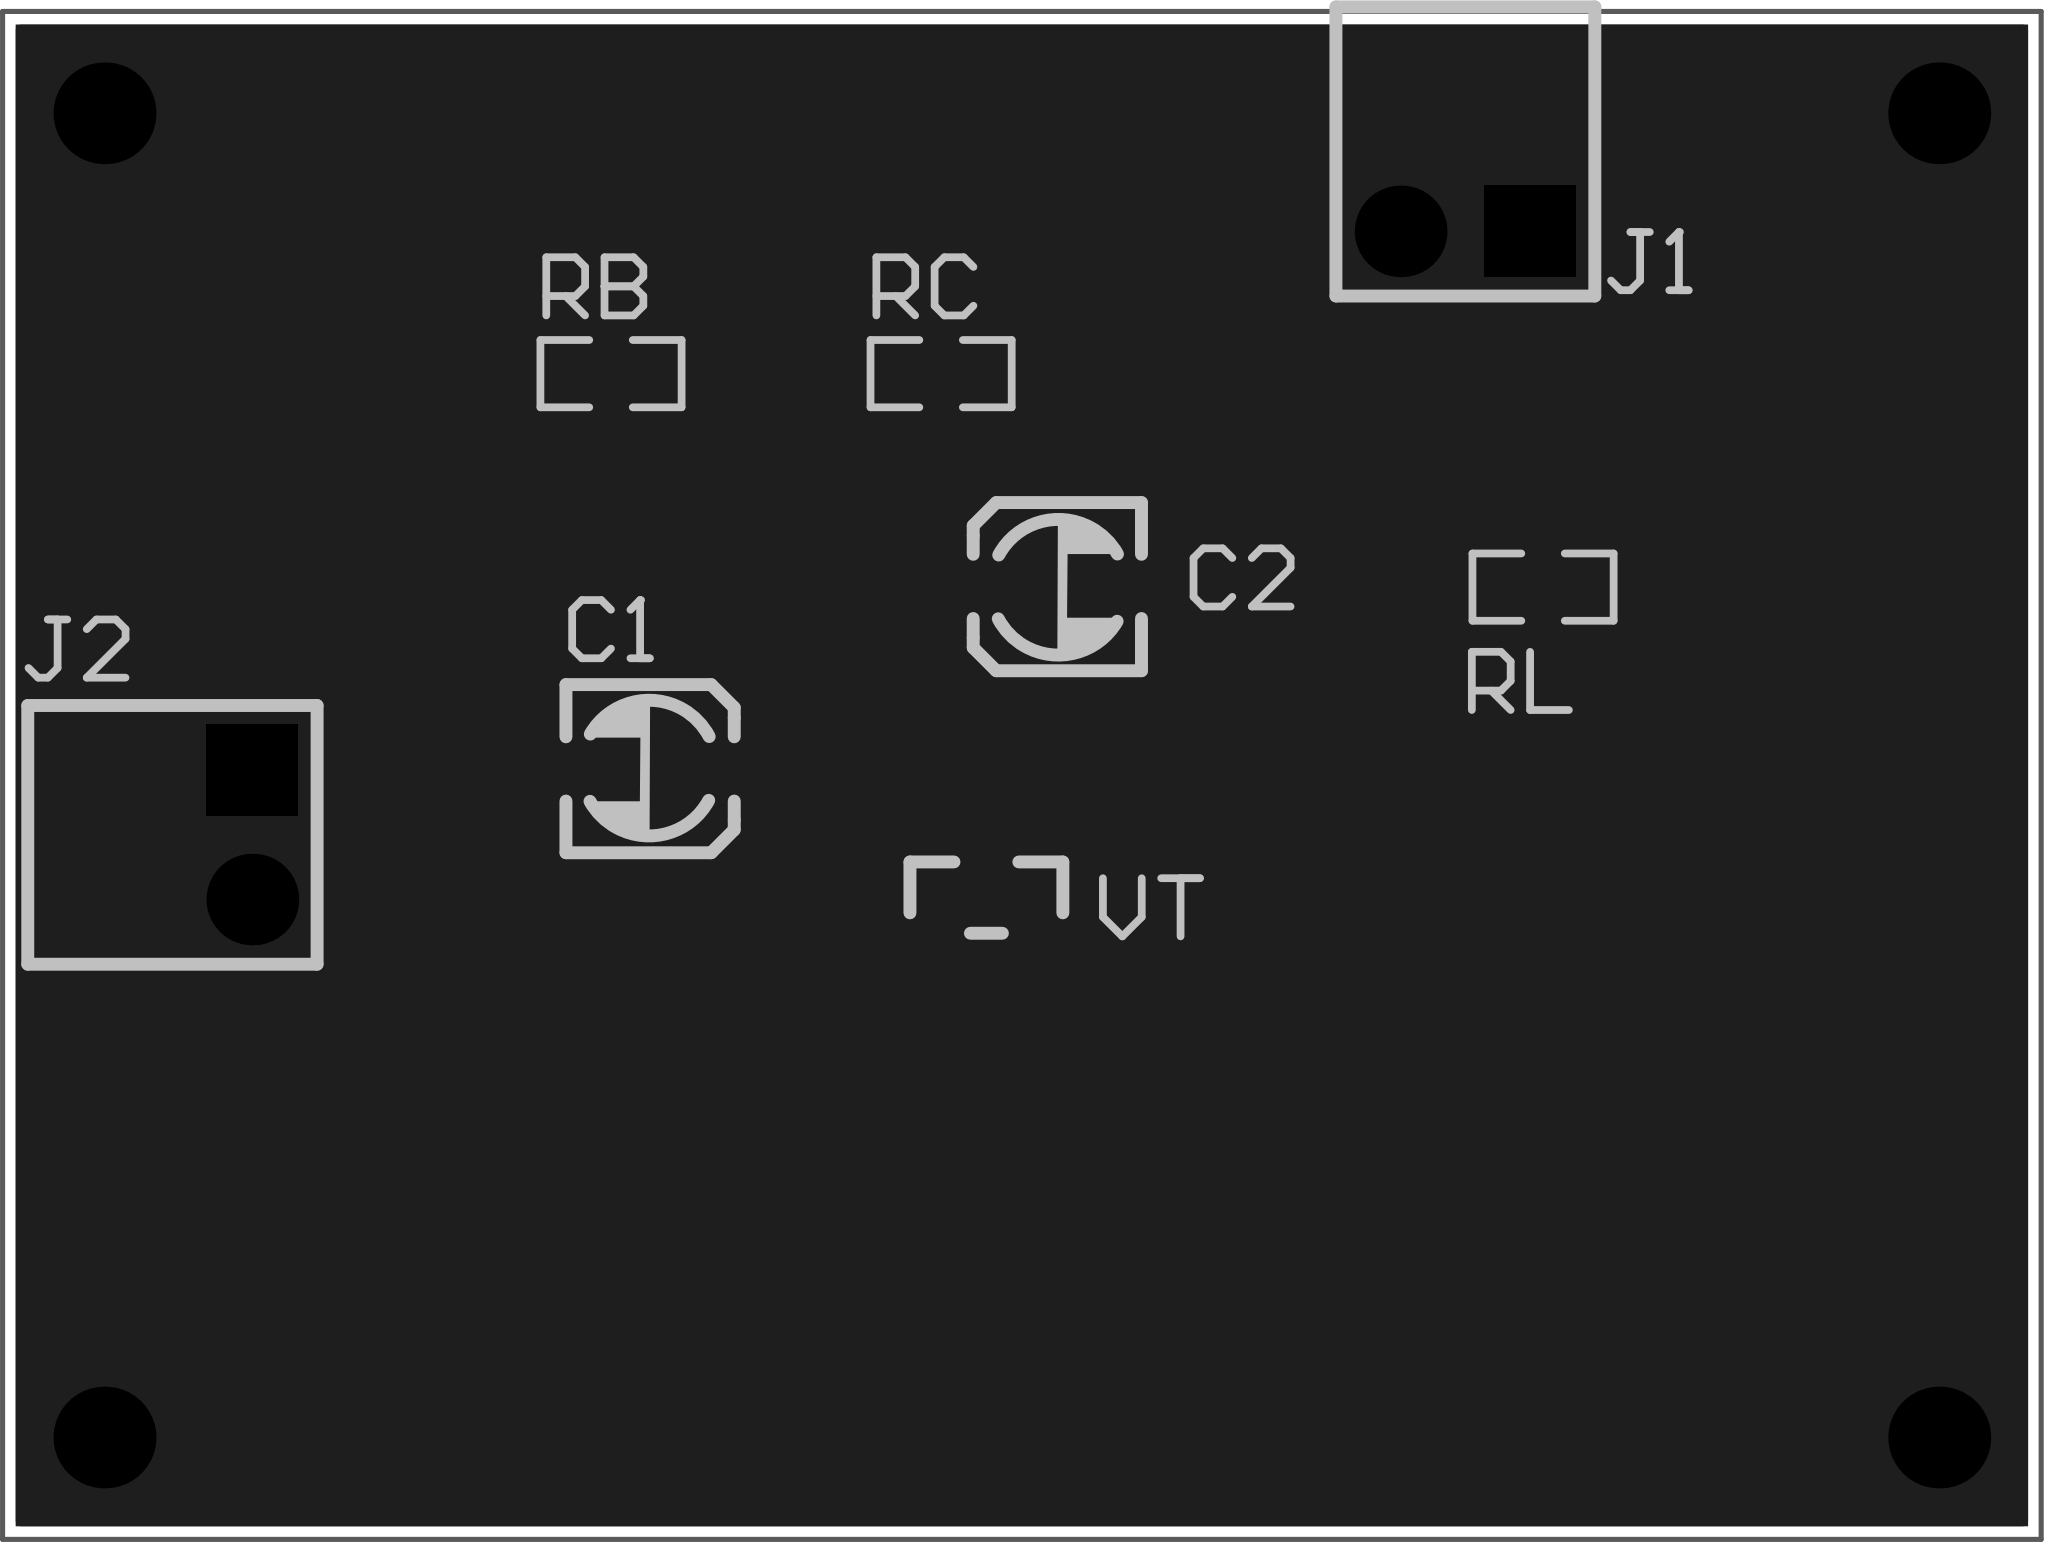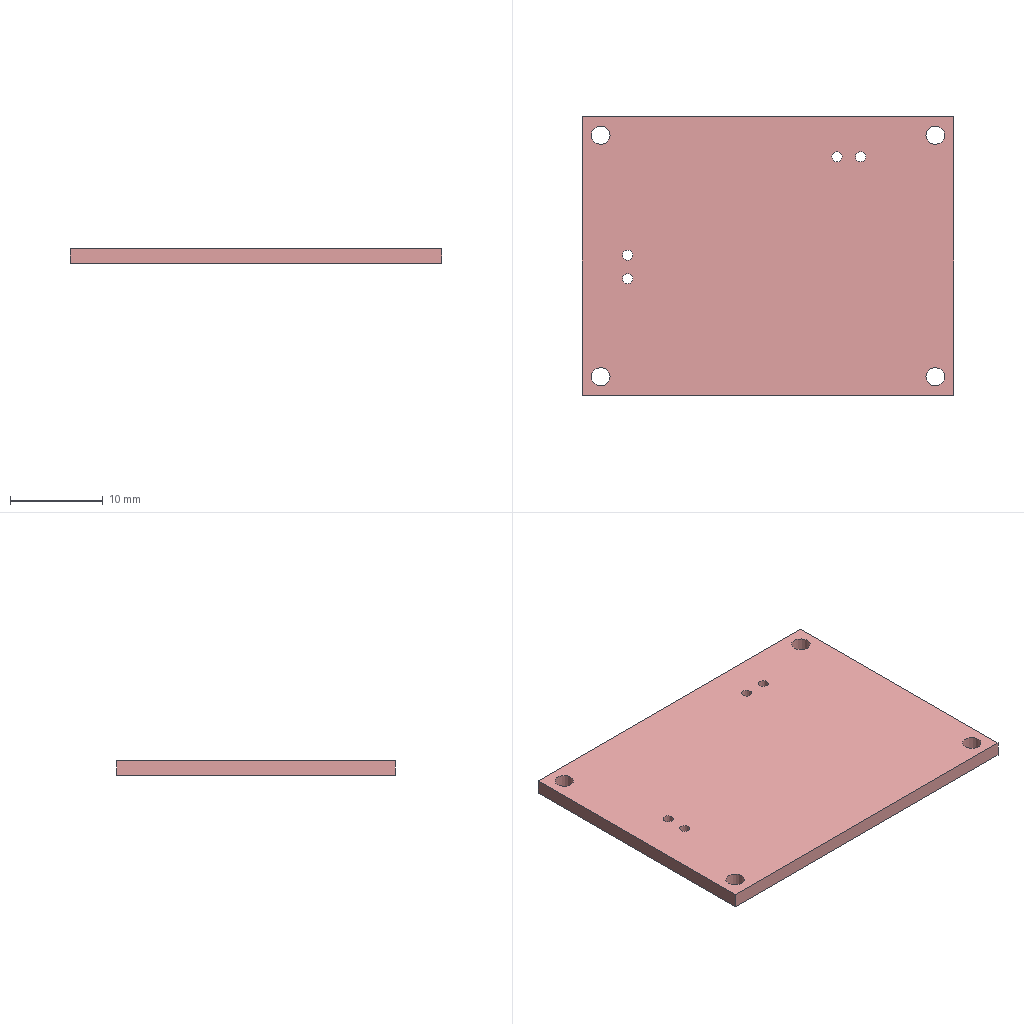Circuit board layout | Altium Designer | box 40 x 30 x 1.6 mm
Layer stack:
# Altium Designer layer stack of  (unit mm; dielectric type: 0 none, 1 core, 2 prepreg, 3 surface material)
index,name,kind,layer,copper_thickness_mm,dielectric_type,dielectric_thickness_mm,dielectric_material,dielectric_constant
0,Top Paste Mask Layer,other,,,,,,
1,Top Silkscreen Layer,other,,,,,,
2,Top Solder Mask Layer,dielectric,,,3,0.01,,3.3
3,Top Layer,copper,Top Layer,0.035,,,,
4,Dielectric1,dielectric,,,3,1.51,FR4,4.5
5,Bottom Layer,copper,Bottom Layer,0.035,,,,
6,Bottom Solder Mask Layer,dielectric,,,3,0.01,,3.3
7,Bottom Silkscreen Layer,other,,,,,,
8,Bottom Paste Mask Layer,other,,,,,,
# drill layer pairs: low layer,high layer
drill_pair,Top Layer,Bottom Layer
Part placement:
Designator,Comment,Layer,Footprint,Center-X(mm),Center-Y(mm),Rotation
J2,,TopLayer,HDR-TH_2P-P2.54-V-M-1,81.101,90.032,270
J1,,TopLayer,HDR-TH_2P-P2.54-V-M-1,104.902,101.882,180
RC,1K,TopLayer,R0603,94.615,99.088,180
RB,5.1K,TopLayer,R0603,88.138,99.088,0
VT,,TopLayer,S8050_SOT-23,95.504,88.801,270
C2,100pF,TopLayer,C_Ele_SMD_3x5.4mm,96.896,94.911,180
C1,100pF,TopLayer,C_Ele_SMD_3x5.4mm,88.905,91.327,0
RL,1K,TopLayer,R0603,106.426,94.897,180
Pad and via stacks:
# Altium Designer via and pad stacks of  (unit mm). Each distinct definition once, with the count of objects using it.
# via: kind,start_layer,end_layer,hole_mm,diameter_mm,mode(0 simple;1 top-mid-bottom;2 full stack),diameter_per_layer,count,example_net
# pad: kind,layer,hole_mm,hole_type(0 round;1 square;2 slot),plating,top_size,top_shape(1 round;2 rect;3 octagon;9 rounded rect),mid_size,bottom_size,mode,footprint,size_per_layer,count,example
pad,Multi-Layer,1.1,0,plated,1.8x1.8,1,1.8x1.8,1.8x1.8,0,HDR-TH_2P-P2.54-V-M-1,,2,J2.2
pad,Multi-Layer,1.1,0,plated,1.8x1.8,2,1.8x1.8,1.8x1.8,0,HDR-TH_2P-P2.54-V-M-1,,2,J2.1
pad,Multi-Layer,2,0,plated,2x2,1,2x2,2x2,0,,,4,1
pad,Top Layer,0,0,plated,0.8065x0.864,2,0.8065x0.864,0.8065x0.864,0,R0603,,6,RC.2
pad,Top Layer,0,0,plated,1x0.8,2,1x0.8,1x0.8,0,S8050_SOT-23,,3,VT.2
pad,Top Layer,0,0,plated,1.999x0.8001,2,1.999x0.8001,1.999x0.8001,0,C_Ele_SMD_3x5.4mm,,4,C2.1
Copper pours:
name,layer,net,type(0 solid;1 hatched;2 none)
Top Layer-GND,Top Layer,GND,0
Bottom Layer-GND,Bottom Layer,GND,0
Design rules, without the lines most boards share:
# Altium Designer design rules of  (exported by Altium Designer, unit mm)
# columns: name | kind | enabled | priority | scope1 | scope2 | descriptor | typed fields (field=value)
creepage | 65 | enabled | 1 | All | All | Creepage Distance Constraint =(0mil) (All),(All) |